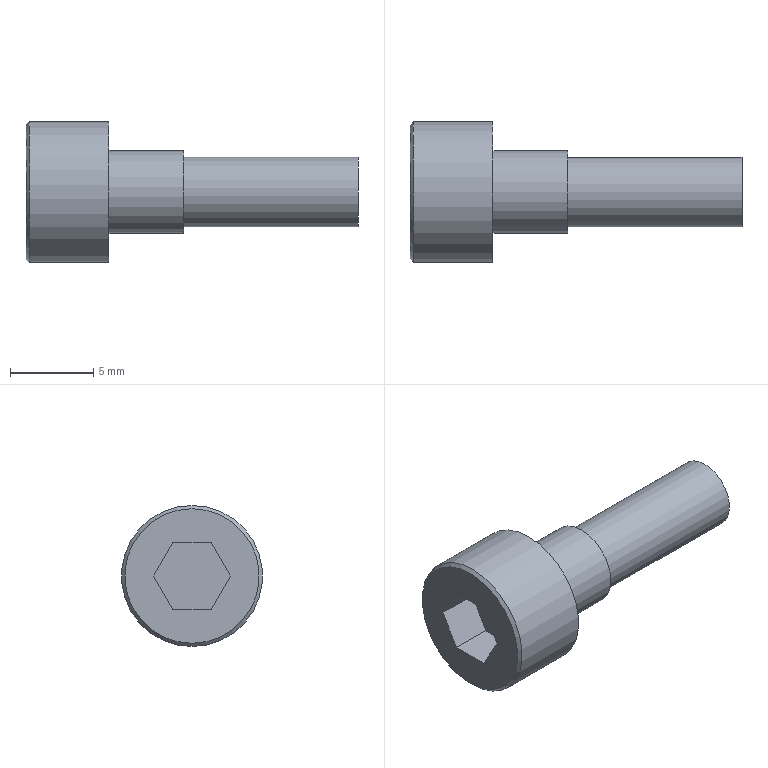Part | STEP file | M3-10_id206_x_t | 1 solid | 15 faces | box 20 x 8.5 x 8.5 mm | volume 482.387 mm3 | plane 11 | cylinder 3 | cone 1 | commonest cylinder face diameters 4.2 x1 5 x1 8.5 x1
STEP:
#1=CARTESIAN_POINT('',(113.,-41.,-17.1));
#2=VERTEX_POINT('',#1);
#3=CARTESIAN_POINT('',(113.,-41.,-15.));
#4=DIRECTION('',(1.,0.,0.));
#5=DIRECTION('',(0.,0.,-1.));
#6=AXIS2_PLACEMENT_3D('',#3,#4,#5);
#7=CIRCLE('',#6,2.1);
#8=EDGE_CURVE('',#2,#2,#7,.T.);
#9=ORIENTED_EDGE('',*,*,#8,.F.);
#10=EDGE_LOOP('',(#9));
#11=FACE_BOUND('',#10,.T.);
#12=CARTESIAN_POINT('',(113.,-41.,-12.5));
#13=VERTEX_POINT('',#12);
#14=CARTESIAN_POINT('',(113.,-41.,-15.));
#15=DIRECTION('',(-1.,0.,0.));
#16=DIRECTION('',(0.,0.,1.));
#17=AXIS2_PLACEMENT_3D('',#14,#15,#16);
#18=CIRCLE('',#17,2.5);
#19=EDGE_CURVE('',#13,#13,#18,.T.);
#20=ORIENTED_EDGE('',*,*,#19,.F.);
#21=EDGE_LOOP('',(#20));
#22=FACE_BOUND('',#21,.T.);
#23=CARTESIAN_POINT('',(113.,-41.,-15.));
#24=DIRECTION('',(1.,0.,0.));
#25=DIRECTION('',(0.,0.,-1.));
#26=AXIS2_PLACEMENT_3D('',#23,#24,#25);
#27=PLANE('',#26);
#28=ADVANCED_FACE('',(#11,#22),#27,.T.);
#29=CARTESIAN_POINT('',(108.5,-41.,-17.5));
#30=VERTEX_POINT('',#29);
#31=CARTESIAN_POINT('',(108.5,-41.,-15.));
#32=DIRECTION('',(-1.,0.,0.));
#33=DIRECTION('',(0.,0.,-1.));
#34=AXIS2_PLACEMENT_3D('',#31,#32,#33);
#35=CIRCLE('',#34,2.5);
#36=EDGE_CURVE('',#30,#30,#35,.T.);
#37=ORIENTED_EDGE('',*,*,#36,.F.);
#38=EDGE_LOOP('',(#37));
#39=FACE_BOUND('',#38,.T.);
#40=ORIENTED_EDGE('',*,*,#19,.T.);
#41=EDGE_LOOP('',(#40));
#42=FACE_BOUND('',#41,.T.);
#43=CARTESIAN_POINT('',(113.,-41.,-15.));
#44=DIRECTION('',(-1.,0.,0.));
#45=DIRECTION('',(0.,0.,1.));
#46=AXIS2_PLACEMENT_3D('',#43,#44,#45);
#47=CYLINDRICAL_SURFACE('',#46,2.5);
#48=ADVANCED_FACE('',(#39,#42),#47,.T.);
#49=CARTESIAN_POINT('',(123.5,-41.,-12.9));
#50=VERTEX_POINT('',#49);
#51=CARTESIAN_POINT('',(123.5,-41.,-15.));
#52=DIRECTION('',(-1.,0.,0.));
#53=DIRECTION('',(0.,0.,1.));
#54=AXIS2_PLACEMENT_3D('',#51,#52,#53);
#55=CIRCLE('',#54,2.1);
#56=EDGE_CURVE('',#50,#50,#55,.T.);
#57=ORIENTED_EDGE('',*,*,#56,.F.);
#58=EDGE_LOOP('',(#57));
#59=FACE_OUTER_BOUND('',#58,.T.);
#60=CARTESIAN_POINT('',(123.5,-41.,-15.));
#61=DIRECTION('',(1.,0.,0.));
#62=DIRECTION('',(0.,0.,-1.));
#63=AXIS2_PLACEMENT_3D('',#60,#61,#62);
#64=PLANE('',#63);
#65=ADVANCED_FACE('',(#59),#64,.T.);
#66=ORIENTED_EDGE('',*,*,#56,.T.);
#67=EDGE_LOOP('',(#66));
#68=FACE_BOUND('',#67,.T.);
#69=ORIENTED_EDGE('',*,*,#8,.T.);
#70=EDGE_LOOP('',(#69));
#71=FACE_BOUND('',#70,.T.);
#72=CARTESIAN_POINT('',(113.,-41.,-15.));
#73=DIRECTION('',(1.,0.,0.));
#74=DIRECTION('',(0.,0.,1.));
#75=AXIS2_PLACEMENT_3D('',#72,#73,#74);
#76=CYLINDRICAL_SURFACE('',#75,2.1);
#77=ADVANCED_FACE('',(#68,#71),#76,.T.);
#78=CARTESIAN_POINT('',(103.5,-39.845,-17.));
#79=VERTEX_POINT('',#78);
#80=CARTESIAN_POINT('',(103.5,-42.155,-17.));
#81=VERTEX_POINT('',#80);
#82=CARTESIAN_POINT('',(103.5,-39.845,-17.));
#83=DIRECTION('',(0.,-1.,0.));
#84=VECTOR('',#83,1.);
#85=LINE('',#82,#84);
#86=EDGE_CURVE('',#79,#81,#85,.T.);
#87=ORIENTED_EDGE('',*,*,#86,.F.);
#88=CARTESIAN_POINT('',(103.5,-38.691,-15.));
#89=VERTEX_POINT('',#88);
#90=CARTESIAN_POINT('',(103.5,-38.691,-15.));
#91=DIRECTION('',(0.,-0.5,-0.866));
#92=VECTOR('',#91,1.);
#93=LINE('',#90,#92);
#94=EDGE_CURVE('',#89,#79,#93,.T.);
#95=ORIENTED_EDGE('',*,*,#94,.F.);
#96=CARTESIAN_POINT('',(103.5,-39.845,-13.));
#97=VERTEX_POINT('',#96);
#98=CARTESIAN_POINT('',(103.5,-39.845,-13.));
#99=DIRECTION('',(0.,0.5,-0.866));
#100=VECTOR('',#99,1.);
#101=LINE('',#98,#100);
#102=EDGE_CURVE('',#97,#89,#101,.T.);
#103=ORIENTED_EDGE('',*,*,#102,.F.);
#104=CARTESIAN_POINT('',(103.5,-42.155,-13.));
#105=VERTEX_POINT('',#104);
#106=CARTESIAN_POINT('',(103.5,-42.155,-13.));
#107=DIRECTION('',(0.,1.,0.));
#108=VECTOR('',#107,1.);
#109=LINE('',#106,#108);
#110=EDGE_CURVE('',#105,#97,#109,.T.);
#111=ORIENTED_EDGE('',*,*,#110,.F.);
#112=CARTESIAN_POINT('',(103.5,-43.309,-15.));
#113=VERTEX_POINT('',#112);
#114=CARTESIAN_POINT('',(103.5,-43.309,-15.));
#115=DIRECTION('',(0.,0.5,0.866));
#116=VECTOR('',#115,1.);
#117=LINE('',#114,#116);
#118=EDGE_CURVE('',#113,#105,#117,.T.);
#119=ORIENTED_EDGE('',*,*,#118,.F.);
#120=CARTESIAN_POINT('',(103.5,-42.155,-17.));
#121=DIRECTION('',(0.,-0.5,0.866));
#122=VECTOR('',#121,1.);
#123=LINE('',#120,#122);
#124=EDGE_CURVE('',#81,#113,#123,.T.);
#125=ORIENTED_EDGE('',*,*,#124,.F.);
#126=EDGE_LOOP('',(#87,#95,#103,#111,#119,#125));
#127=FACE_BOUND('',#126,.T.);
#128=CARTESIAN_POINT('',(103.5,-41.,-10.95));
#129=VERTEX_POINT('',#128);
#130=CARTESIAN_POINT('',(103.5,-41.,-15.));
#131=DIRECTION('',(-1.,0.,0.));
#132=DIRECTION('',(0.,0.,1.));
#133=AXIS2_PLACEMENT_3D('',#130,#131,#132);
#134=CIRCLE('',#133,4.05);
#135=EDGE_CURVE('',#129,#129,#134,.T.);
#136=ORIENTED_EDGE('',*,*,#135,.T.);
#137=EDGE_LOOP('',(#136));
#138=FACE_BOUND('',#137,.T.);
#139=CARTESIAN_POINT('',(103.5,-41.,-15.));
#140=DIRECTION('',(-1.,0.,0.));
#141=DIRECTION('',(0.,0.,1.));
#142=AXIS2_PLACEMENT_3D('',#139,#140,#141);
#143=PLANE('',#142);
#144=ADVANCED_FACE('',(#127,#138),#143,.T.);
#145=ORIENTED_EDGE('',*,*,#36,.T.);
#146=EDGE_LOOP('',(#145));
#147=FACE_BOUND('',#146,.T.);
#148=CARTESIAN_POINT('',(108.5,-41.,-10.75));
#149=VERTEX_POINT('',#148);
#150=CARTESIAN_POINT('',(108.5,-41.,-15.));
#151=DIRECTION('',(-1.,0.,0.));
#152=DIRECTION('',(0.,0.,1.));
#153=AXIS2_PLACEMENT_3D('',#150,#151,#152);
#154=CIRCLE('',#153,4.25);
#155=EDGE_CURVE('',#149,#149,#154,.T.);
#156=ORIENTED_EDGE('',*,*,#155,.F.);
#157=EDGE_LOOP('',(#156));
#158=FACE_BOUND('',#157,.T.);
#159=CARTESIAN_POINT('',(108.5,-41.,-15.));
#160=DIRECTION('',(1.,0.,0.));
#161=DIRECTION('',(0.,0.,-1.));
#162=AXIS2_PLACEMENT_3D('',#159,#160,#161);
#163=PLANE('',#162);
#164=ADVANCED_FACE('',(#147,#158),#163,.T.);
#165=CARTESIAN_POINT('',(103.7,-41.,-10.75));
#166=VERTEX_POINT('',#165);
#167=CARTESIAN_POINT('',(103.7,-41.,-15.));
#168=DIRECTION('',(1.,0.,0.));
#169=DIRECTION('',(0.,0.,1.));
#170=AXIS2_PLACEMENT_3D('',#167,#168,#169);
#171=CIRCLE('',#170,4.25);
#172=EDGE_CURVE('',#166,#166,#171,.T.);
#173=ORIENTED_EDGE('',*,*,#172,.T.);
#174=EDGE_LOOP('',(#173));
#175=FACE_BOUND('',#174,.T.);
#176=ORIENTED_EDGE('',*,*,#155,.T.);
#177=EDGE_LOOP('',(#176));
#178=FACE_BOUND('',#177,.T.);
#179=CARTESIAN_POINT('',(108.5,-41.,-15.));
#180=DIRECTION('',(-1.,0.,0.));
#181=DIRECTION('',(0.,0.,1.));
#182=AXIS2_PLACEMENT_3D('',#179,#180,#181);
#183=CYLINDRICAL_SURFACE('',#182,4.25);
#184=ADVANCED_FACE('',(#175,#178),#183,.T.);
#185=ORIENTED_EDGE('',*,*,#135,.F.);
#186=EDGE_LOOP('',(#185));
#187=FACE_BOUND('',#186,.T.);
#188=ORIENTED_EDGE('',*,*,#172,.F.);
#189=EDGE_LOOP('',(#188));
#190=FACE_BOUND('',#189,.T.);
#191=CARTESIAN_POINT('',(103.7,-41.,-15.));
#192=DIRECTION('',(1.,0.,0.));
#193=DIRECTION('',(0.,0.,-1.));
#194=AXIS2_PLACEMENT_3D('',#191,#192,#193);
#195=CONICAL_SURFACE('',#194,4.25,45.);
#196=ADVANCED_FACE('',(#187,#190),#195,.T.);
#197=ORIENTED_EDGE('',*,*,#86,.T.);
#198=CARTESIAN_POINT('',(106.,-42.155,-17.));
#199=VERTEX_POINT('',#198);
#200=CARTESIAN_POINT('',(106.,-42.155,-17.));
#201=DIRECTION('',(1.,0.,0.));
#202=VECTOR('',#201,1.);
#203=LINE('',#200,#202);
#204=EDGE_CURVE('',#81,#199,#203,.T.);
#205=ORIENTED_EDGE('',*,*,#204,.T.);
#206=CARTESIAN_POINT('',(106.,-39.845,-17.));
#207=VERTEX_POINT('',#206);
#208=CARTESIAN_POINT('',(106.,-39.845,-17.));
#209=DIRECTION('',(0.,1.,0.));
#210=VECTOR('',#209,1.);
#211=LINE('',#208,#210);
#212=EDGE_CURVE('',#199,#207,#211,.T.);
#213=ORIENTED_EDGE('',*,*,#212,.T.);
#214=CARTESIAN_POINT('',(106.,-39.845,-17.));
#215=DIRECTION('',(1.,0.,0.));
#216=VECTOR('',#215,1.);
#217=LINE('',#214,#216);
#218=EDGE_CURVE('',#79,#207,#217,.T.);
#219=ORIENTED_EDGE('',*,*,#218,.F.);
#220=EDGE_LOOP('',(#197,#205,#213,#219));
#221=FACE_OUTER_BOUND('',#220,.T.);
#222=CARTESIAN_POINT('',(106.,-39.845,-17.));
#223=DIRECTION('',(0.,0.,-1.));
#224=DIRECTION('',(0.,-1.,0.));
#225=AXIS2_PLACEMENT_3D('',#222,#223,#224);
#226=PLANE('',#225);
#227=ADVANCED_FACE('',(#221),#226,.F.);
#228=ORIENTED_EDGE('',*,*,#124,.T.);
#229=CARTESIAN_POINT('',(106.,-43.309,-15.));
#230=VERTEX_POINT('',#229);
#231=CARTESIAN_POINT('',(106.,-43.309,-15.));
#232=DIRECTION('',(1.,0.,0.));
#233=VECTOR('',#232,1.);
#234=LINE('',#231,#233);
#235=EDGE_CURVE('',#113,#230,#234,.T.);
#236=ORIENTED_EDGE('',*,*,#235,.T.);
#237=CARTESIAN_POINT('',(106.,-42.155,-17.));
#238=DIRECTION('',(0.,0.5,-0.866));
#239=VECTOR('',#238,1.);
#240=LINE('',#237,#239);
#241=EDGE_CURVE('',#230,#199,#240,.T.);
#242=ORIENTED_EDGE('',*,*,#241,.T.);
#243=ORIENTED_EDGE('',*,*,#204,.F.);
#244=EDGE_LOOP('',(#228,#236,#242,#243));
#245=FACE_OUTER_BOUND('',#244,.T.);
#246=CARTESIAN_POINT('',(106.,-42.155,-17.));
#247=DIRECTION('',(0.,-0.866,-0.5));
#248=DIRECTION('',(0.,-0.5,0.866));
#249=AXIS2_PLACEMENT_3D('',#246,#247,#248);
#250=PLANE('',#249);
#251=ADVANCED_FACE('',(#245),#250,.F.);
#252=ORIENTED_EDGE('',*,*,#118,.T.);
#253=CARTESIAN_POINT('',(106.,-42.155,-13.));
#254=VERTEX_POINT('',#253);
#255=CARTESIAN_POINT('',(106.,-42.155,-13.));
#256=DIRECTION('',(1.,0.,0.));
#257=VECTOR('',#256,1.);
#258=LINE('',#255,#257);
#259=EDGE_CURVE('',#105,#254,#258,.T.);
#260=ORIENTED_EDGE('',*,*,#259,.T.);
#261=CARTESIAN_POINT('',(106.,-43.309,-15.));
#262=DIRECTION('',(0.,-0.5,-0.866));
#263=VECTOR('',#262,1.);
#264=LINE('',#261,#263);
#265=EDGE_CURVE('',#254,#230,#264,.T.);
#266=ORIENTED_EDGE('',*,*,#265,.T.);
#267=ORIENTED_EDGE('',*,*,#235,.F.);
#268=EDGE_LOOP('',(#252,#260,#266,#267));
#269=FACE_OUTER_BOUND('',#268,.T.);
#270=CARTESIAN_POINT('',(106.,-43.309,-15.));
#271=DIRECTION('',(0.,-0.866,0.5));
#272=DIRECTION('',(0.,0.5,0.866));
#273=AXIS2_PLACEMENT_3D('',#270,#271,#272);
#274=PLANE('',#273);
#275=ADVANCED_FACE('',(#269),#274,.F.);
#276=ORIENTED_EDGE('',*,*,#110,.T.);
#277=CARTESIAN_POINT('',(106.,-39.845,-13.));
#278=VERTEX_POINT('',#277);
#279=CARTESIAN_POINT('',(106.,-39.845,-13.));
#280=DIRECTION('',(1.,0.,0.));
#281=VECTOR('',#280,1.);
#282=LINE('',#279,#281);
#283=EDGE_CURVE('',#97,#278,#282,.T.);
#284=ORIENTED_EDGE('',*,*,#283,.T.);
#285=CARTESIAN_POINT('',(106.,-42.155,-13.));
#286=DIRECTION('',(0.,-1.,0.));
#287=VECTOR('',#286,1.);
#288=LINE('',#285,#287);
#289=EDGE_CURVE('',#278,#254,#288,.T.);
#290=ORIENTED_EDGE('',*,*,#289,.T.);
#291=ORIENTED_EDGE('',*,*,#259,.F.);
#292=EDGE_LOOP('',(#276,#284,#290,#291));
#293=FACE_OUTER_BOUND('',#292,.T.);
#294=CARTESIAN_POINT('',(106.,-42.155,-13.));
#295=DIRECTION('',(0.,0.,1.));
#296=DIRECTION('',(0.,1.,0.));
#297=AXIS2_PLACEMENT_3D('',#294,#295,#296);
#298=PLANE('',#297);
#299=ADVANCED_FACE('',(#293),#298,.F.);
#300=ORIENTED_EDGE('',*,*,#102,.T.);
#301=CARTESIAN_POINT('',(106.,-38.691,-15.));
#302=VERTEX_POINT('',#301);
#303=CARTESIAN_POINT('',(106.,-38.691,-15.));
#304=DIRECTION('',(1.,0.,0.));
#305=VECTOR('',#304,1.);
#306=LINE('',#303,#305);
#307=EDGE_CURVE('',#89,#302,#306,.T.);
#308=ORIENTED_EDGE('',*,*,#307,.T.);
#309=CARTESIAN_POINT('',(106.,-39.845,-13.));
#310=DIRECTION('',(0.,-0.5,0.866));
#311=VECTOR('',#310,1.);
#312=LINE('',#309,#311);
#313=EDGE_CURVE('',#302,#278,#312,.T.);
#314=ORIENTED_EDGE('',*,*,#313,.T.);
#315=ORIENTED_EDGE('',*,*,#283,.F.);
#316=EDGE_LOOP('',(#300,#308,#314,#315));
#317=FACE_OUTER_BOUND('',#316,.T.);
#318=CARTESIAN_POINT('',(106.,-39.845,-13.));
#319=DIRECTION('',(0.,0.866,0.5));
#320=DIRECTION('',(0.,0.5,-0.866));
#321=AXIS2_PLACEMENT_3D('',#318,#319,#320);
#322=PLANE('',#321);
#323=ADVANCED_FACE('',(#317),#322,.F.);
#324=ORIENTED_EDGE('',*,*,#94,.T.);
#325=ORIENTED_EDGE('',*,*,#218,.T.);
#326=CARTESIAN_POINT('',(106.,-38.691,-15.));
#327=DIRECTION('',(0.,0.5,0.866));
#328=VECTOR('',#327,1.);
#329=LINE('',#326,#328);
#330=EDGE_CURVE('',#207,#302,#329,.T.);
#331=ORIENTED_EDGE('',*,*,#330,.T.);
#332=ORIENTED_EDGE('',*,*,#307,.F.);
#333=EDGE_LOOP('',(#324,#325,#331,#332));
#334=FACE_OUTER_BOUND('',#333,.T.);
#335=CARTESIAN_POINT('',(106.,-38.691,-15.));
#336=DIRECTION('',(0.,0.866,-0.5));
#337=DIRECTION('',(0.,-0.5,-0.866));
#338=AXIS2_PLACEMENT_3D('',#335,#336,#337);
#339=PLANE('',#338);
#340=ADVANCED_FACE('',(#334),#339,.F.);
#341=ORIENTED_EDGE('',*,*,#212,.F.);
#342=ORIENTED_EDGE('',*,*,#241,.F.);
#343=ORIENTED_EDGE('',*,*,#265,.F.);
#344=ORIENTED_EDGE('',*,*,#289,.F.);
#345=ORIENTED_EDGE('',*,*,#313,.F.);
#346=ORIENTED_EDGE('',*,*,#330,.F.);
#347=EDGE_LOOP('',(#341,#342,#343,#344,#345,#346));
#348=FACE_OUTER_BOUND('',#347,.T.);
#349=CARTESIAN_POINT('',(106.,-41.,-15.));
#350=DIRECTION('',(-1.,0.,0.));
#351=DIRECTION('',(0.,0.,1.));
#352=AXIS2_PLACEMENT_3D('',#349,#350,#351);
#353=PLANE('',#352);
#354=ADVANCED_FACE('',(#348),#353,.T.);
#355=CLOSED_SHELL('',(#28,#48,#65,#77,#144,#164,#184,#196,#227,#251,#275,#299,#323,#340,#354));
#356=MANIFOLD_SOLID_BREP('',#355);
#357=(LENGTH_UNIT()NAMED_UNIT(*)SI_UNIT(.MILLI.,.METRE.));
#358=UNCERTAINTY_MEASURE_WITH_UNIT(LENGTH_MEASURE(0.00002),#357,'','');
#359=(NAMED_UNIT(*)PLANE_ANGLE_UNIT()SI_UNIT($,.RADIAN.));
#360=PLANE_ANGLE_MEASURE_WITH_UNIT(PLANE_ANGLE_MEASURE(0.01745),#359);
#361=DIMENSIONAL_EXPONENTS(0.,0.,0.,0.,0.,0.,0.);
#362=(CONVERSION_BASED_UNIT('DEGREE',#360)NAMED_UNIT(#361)PLANE_ANGLE_UNIT());
#363=(NAMED_UNIT(*)SI_UNIT($,.STERADIAN.)SOLID_ANGLE_UNIT());
#364=(GEOMETRIC_REPRESENTATION_CONTEXT(3)GLOBAL_UNCERTAINTY_ASSIGNED_CONTEXT((#358))GLOBAL_UNIT_ASSIGNED_CONTEXT((#357,#362,#363))REPRESENTATION_CONTEXT('',''));
#365=ADVANCED_BREP_SHAPE_REPRESENTATION('',(#356),#364);